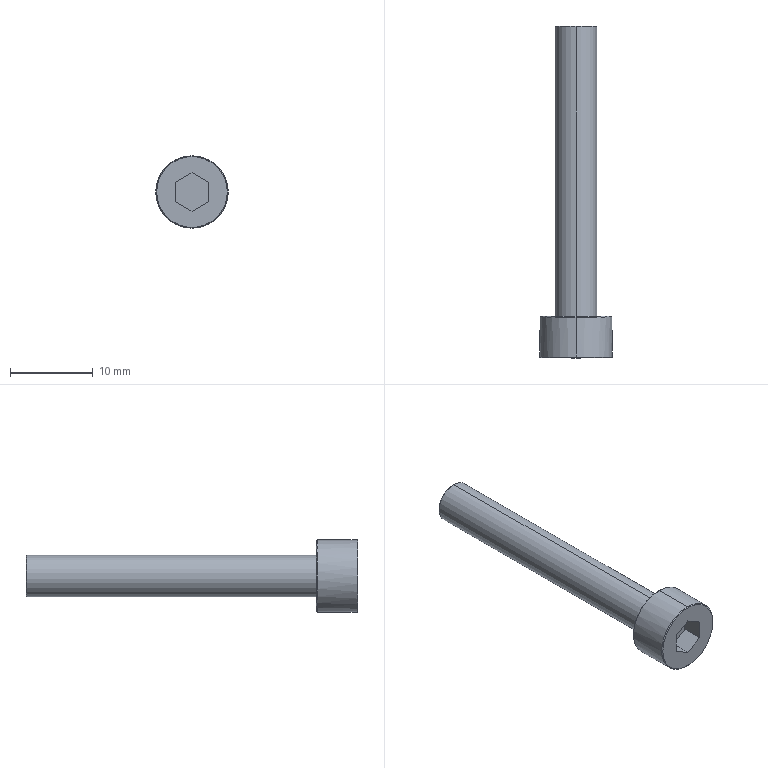Part | SolidWorks | features BaseBody 1 | 1 solid | 20 faces | box 8.72 x 40 x 8.72 mm | volume 950.488 mm3 | plane 10 | cone 6 | cylinder 4 | commonest cylinder face diameters 5 x2 8.72 x2
STEP:
#1=CARTESIAN_POINT('',(0.,39.9,-2.5));
#2=VERTEX_POINT('',#1);
#3=CARTESIAN_POINT('',(0.,39.9,2.5));
#4=VERTEX_POINT('',#3);
#5=CARTESIAN_POINT('',(0.,39.9,0.));
#6=DIRECTION('',(0.,-1.,0.));
#7=DIRECTION('',(0.,0.,-1.));
#8=AXIS2_PLACEMENT_3D('',#5,#6,#7);
#9=CIRCLE('',#8,2.5);
#10=EDGE_CURVE('',#2,#4,#9,.T.);
#11=ORIENTED_EDGE('',*,*,#10,.T.);
#12=CARTESIAN_POINT('',(0.,5.,2.5));
#13=VERTEX_POINT('',#12);
#14=CARTESIAN_POINT('',(0.,40.,2.5));
#15=DIRECTION('',(0.,-1.,0.));
#16=VECTOR('',#15,1000.);
#17=LINE('',#14,#16);
#18=EDGE_CURVE('',#4,#13,#17,.T.);
#19=ORIENTED_EDGE('',*,*,#18,.T.);
#20=CARTESIAN_POINT('',(0.,5.,-2.5));
#21=VERTEX_POINT('',#20);
#22=CARTESIAN_POINT('',(0.,5.,0.));
#23=DIRECTION('',(0.,1.,0.));
#24=DIRECTION('',(0.,0.,-1.));
#25=AXIS2_PLACEMENT_3D('',#22,#23,#24);
#26=CIRCLE('',#25,2.5);
#27=EDGE_CURVE('',#13,#21,#26,.T.);
#28=ORIENTED_EDGE('',*,*,#27,.T.);
#29=CARTESIAN_POINT('',(0.,40.,-2.5));
#30=DIRECTION('',(0.,-1.,0.));
#31=VECTOR('',#30,1000.);
#32=LINE('',#29,#31);
#33=EDGE_CURVE('',#2,#21,#32,.T.);
#34=ORIENTED_EDGE('',*,*,#33,.F.);
#35=EDGE_LOOP('',(#11,#19,#28,#34));
#36=FACE_OUTER_BOUND('',#35,.T.);
#37=CARTESIAN_POINT('',(0.,40.,0.));
#38=DIRECTION('',(0.,-1.,0.));
#39=DIRECTION('',(0.,0.,-1.));
#40=AXIS2_PLACEMENT_3D('',#37,#38,#39);
#41=CYLINDRICAL_SURFACE('',#40,2.5);
#42=ADVANCED_FACE('',(#36),#41,.T.);
#43=CARTESIAN_POINT('',(0.,40.,-2.4));
#44=VERTEX_POINT('',#43);
#45=CARTESIAN_POINT('',(0.,40.,2.4));
#46=VERTEX_POINT('',#45);
#47=CARTESIAN_POINT('',(0.,40.,0.));
#48=DIRECTION('',(0.,-1.,0.));
#49=DIRECTION('',(0.,0.,-1.));
#50=AXIS2_PLACEMENT_3D('',#47,#48,#49);
#51=CIRCLE('',#50,2.4);
#52=EDGE_CURVE('',#44,#46,#51,.T.);
#53=ORIENTED_EDGE('',*,*,#52,.T.);
#54=CARTESIAN_POINT('',(0.,39.9,2.5));
#55=DIRECTION('',(0.,-0.7071,0.7071));
#56=VECTOR('',#55,1000.);
#57=LINE('',#54,#56);
#58=EDGE_CURVE('',#46,#4,#57,.T.);
#59=ORIENTED_EDGE('',*,*,#58,.T.);
#60=ORIENTED_EDGE('',*,*,#10,.F.);
#61=CARTESIAN_POINT('',(0.,39.9,-2.5));
#62=DIRECTION('',(0.,-0.7071,-0.7071));
#63=VECTOR('',#62,1000.);
#64=LINE('',#61,#63);
#65=EDGE_CURVE('',#44,#2,#64,.T.);
#66=ORIENTED_EDGE('',*,*,#65,.F.);
#67=EDGE_LOOP('',(#53,#59,#60,#66));
#68=FACE_OUTER_BOUND('',#67,.T.);
#69=CARTESIAN_POINT('',(0.,39.9,0.));
#70=DIRECTION('',(0.,-1.,0.));
#71=DIRECTION('',(0.,0.,-1.));
#72=AXIS2_PLACEMENT_3D('',#69,#70,#71);
#73=CONICAL_SURFACE('',#72,2.5,0.7854);
#74=ADVANCED_FACE('',(#68),#73,.T.);
#75=CARTESIAN_POINT('',(0.,5.,4.26));
#76=VERTEX_POINT('',#75);
#77=CARTESIAN_POINT('',(0.,5.,-4.26));
#78=VERTEX_POINT('',#77);
#79=CARTESIAN_POINT('',(0.,5.,0.));
#80=DIRECTION('',(0.,1.,0.));
#81=DIRECTION('',(0.,0.,-1.));
#82=AXIS2_PLACEMENT_3D('',#79,#80,#81);
#83=CIRCLE('',#82,4.26);
#84=EDGE_CURVE('',#76,#78,#83,.T.);
#85=ORIENTED_EDGE('',*,*,#84,.F.);
#86=CARTESIAN_POINT('',(0.,4.9,4.36));
#87=VERTEX_POINT('',#86);
#88=CARTESIAN_POINT('',(0.,4.9,4.36));
#89=DIRECTION('',(0.,-0.7071,0.7071));
#90=VECTOR('',#89,1000.);
#91=LINE('',#88,#90);
#92=EDGE_CURVE('',#76,#87,#91,.T.);
#93=ORIENTED_EDGE('',*,*,#92,.T.);
#94=CARTESIAN_POINT('',(0.,4.9,-4.36));
#95=VERTEX_POINT('',#94);
#96=CARTESIAN_POINT('',(0.,4.9,0.));
#97=DIRECTION('',(0.,1.,0.));
#98=DIRECTION('',(0.,0.,-1.));
#99=AXIS2_PLACEMENT_3D('',#96,#97,#98);
#100=CIRCLE('',#99,4.36);
#101=EDGE_CURVE('',#87,#95,#100,.T.);
#102=ORIENTED_EDGE('',*,*,#101,.T.);
#103=CARTESIAN_POINT('',(0.,4.9,-4.36));
#104=DIRECTION('',(0.,-0.7071,-0.7071));
#105=VECTOR('',#104,1000.);
#106=LINE('',#103,#105);
#107=EDGE_CURVE('',#78,#95,#106,.T.);
#108=ORIENTED_EDGE('',*,*,#107,.F.);
#109=EDGE_LOOP('',(#85,#93,#102,#108));
#110=FACE_OUTER_BOUND('',#109,.T.);
#111=CARTESIAN_POINT('',(0.,4.9,0.));
#112=DIRECTION('',(0.,-1.,0.));
#113=DIRECTION('',(0.,0.,-1.));
#114=AXIS2_PLACEMENT_3D('',#111,#112,#113);
#115=CONICAL_SURFACE('',#114,4.36,0.7854);
#116=ADVANCED_FACE('',(#110),#115,.T.);
#117=ORIENTED_EDGE('',*,*,#101,.F.);
#118=CARTESIAN_POINT('',(0.,0.1,4.36));
#119=VERTEX_POINT('',#118);
#120=CARTESIAN_POINT('',(0.,5.,4.36));
#121=DIRECTION('',(0.,-1.,0.));
#122=VECTOR('',#121,1000.);
#123=LINE('',#120,#122);
#124=EDGE_CURVE('',#87,#119,#123,.T.);
#125=ORIENTED_EDGE('',*,*,#124,.T.);
#126=CARTESIAN_POINT('',(4.36,0.1,0.));
#127=VERTEX_POINT('',#126);
#128=CARTESIAN_POINT('',(0.,0.1,0.));
#129=DIRECTION('',(0.,1.,0.));
#130=DIRECTION('',(0.,0.,-1.));
#131=AXIS2_PLACEMENT_3D('',#128,#129,#130);
#132=CIRCLE('',#131,4.36);
#133=EDGE_CURVE('',#119,#127,#132,.T.);
#134=ORIENTED_EDGE('',*,*,#133,.T.);
#135=CARTESIAN_POINT('',(0.,0.1,-4.36));
#136=VERTEX_POINT('',#135);
#137=CARTESIAN_POINT('',(0.,0.1,0.));
#138=DIRECTION('',(0.,1.,0.));
#139=DIRECTION('',(0.,0.,-1.));
#140=AXIS2_PLACEMENT_3D('',#137,#138,#139);
#141=CIRCLE('',#140,4.36);
#142=EDGE_CURVE('',#127,#136,#141,.T.);
#143=ORIENTED_EDGE('',*,*,#142,.T.);
#144=CARTESIAN_POINT('',(0.,5.,-4.36));
#145=DIRECTION('',(0.,-1.,0.));
#146=VECTOR('',#145,1000.);
#147=LINE('',#144,#146);
#148=EDGE_CURVE('',#95,#136,#147,.T.);
#149=ORIENTED_EDGE('',*,*,#148,.F.);
#150=EDGE_LOOP('',(#117,#125,#134,#143,#149));
#151=FACE_OUTER_BOUND('',#150,.T.);
#152=CARTESIAN_POINT('',(0.,5.,0.));
#153=DIRECTION('',(0.,-1.,0.));
#154=DIRECTION('',(0.,0.,-1.));
#155=AXIS2_PLACEMENT_3D('',#152,#153,#154);
#156=CYLINDRICAL_SURFACE('',#155,4.36);
#157=ADVANCED_FACE('',(#151),#156,.T.);
#158=CARTESIAN_POINT('',(-4.26,0.,0.));
#159=VERTEX_POINT('',#158);
#160=CARTESIAN_POINT('',(4.26,0.,0.));
#161=VERTEX_POINT('',#160);
#162=CARTESIAN_POINT('',(0.,0.,0.));
#163=DIRECTION('',(0.,1.,0.));
#164=DIRECTION('',(-1.,0.,0.));
#165=AXIS2_PLACEMENT_3D('',#162,#163,#164);
#166=CIRCLE('',#165,4.26);
#167=EDGE_CURVE('',#159,#161,#166,.T.);
#168=ORIENTED_EDGE('',*,*,#167,.T.);
#169=CARTESIAN_POINT('',(4.36,0.1,0.));
#170=DIRECTION('',(0.7071,0.7071,0.));
#171=VECTOR('',#170,1000.);
#172=LINE('',#169,#171);
#173=EDGE_CURVE('',#161,#127,#172,.T.);
#174=ORIENTED_EDGE('',*,*,#173,.T.);
#175=ORIENTED_EDGE('',*,*,#133,.F.);
#176=CARTESIAN_POINT('',(-4.36,0.1,0.));
#177=VERTEX_POINT('',#176);
#178=CARTESIAN_POINT('',(0.,0.1,0.));
#179=DIRECTION('',(0.,1.,0.));
#180=DIRECTION('',(0.,0.,-1.));
#181=AXIS2_PLACEMENT_3D('',#178,#179,#180);
#182=CIRCLE('',#181,4.36);
#183=EDGE_CURVE('',#177,#119,#182,.T.);
#184=ORIENTED_EDGE('',*,*,#183,.F.);
#185=CARTESIAN_POINT('',(-4.36,0.1,0.));
#186=DIRECTION('',(-0.7071,0.7071,0.));
#187=VECTOR('',#186,1000.);
#188=LINE('',#185,#187);
#189=EDGE_CURVE('',#159,#177,#188,.T.);
#190=ORIENTED_EDGE('',*,*,#189,.F.);
#191=EDGE_LOOP('',(#168,#174,#175,#184,#190));
#192=FACE_OUTER_BOUND('',#191,.T.);
#193=CARTESIAN_POINT('',(0.,0.1,0.));
#194=DIRECTION('',(0.,1.,0.));
#195=DIRECTION('',(-1.,0.,0.));
#196=AXIS2_PLACEMENT_3D('',#193,#194,#195);
#197=CONICAL_SURFACE('',#196,4.36,0.7854);
#198=ADVANCED_FACE('',(#192),#197,.T.);
#199=ORIENTED_EDGE('',*,*,#18,.F.);
#200=CARTESIAN_POINT('',(0.,39.9,0.));
#201=DIRECTION('',(0.,-1.,0.));
#202=DIRECTION('',(0.,0.,-1.));
#203=AXIS2_PLACEMENT_3D('',#200,#201,#202);
#204=CIRCLE('',#203,2.5);
#205=EDGE_CURVE('',#4,#2,#204,.T.);
#206=ORIENTED_EDGE('',*,*,#205,.T.);
#207=ORIENTED_EDGE('',*,*,#33,.T.);
#208=CARTESIAN_POINT('',(0.,5.,0.));
#209=DIRECTION('',(0.,1.,0.));
#210=DIRECTION('',(0.,0.,-1.));
#211=AXIS2_PLACEMENT_3D('',#208,#209,#210);
#212=CIRCLE('',#211,2.5);
#213=EDGE_CURVE('',#21,#13,#212,.T.);
#214=ORIENTED_EDGE('',*,*,#213,.T.);
#215=EDGE_LOOP('',(#199,#206,#207,#214));
#216=FACE_OUTER_BOUND('',#215,.T.);
#217=CARTESIAN_POINT('',(0.,40.,0.));
#218=DIRECTION('',(0.,-1.,0.));
#219=DIRECTION('',(0.,0.,-1.));
#220=AXIS2_PLACEMENT_3D('',#217,#218,#219);
#221=CYLINDRICAL_SURFACE('',#220,2.5);
#222=ADVANCED_FACE('',(#216),#221,.T.);
#223=ORIENTED_EDGE('',*,*,#213,.F.);
#224=ORIENTED_EDGE('',*,*,#27,.F.);
#225=EDGE_LOOP('',(#223,#224));
#226=FACE_BOUND('',#225,.T.);
#227=CARTESIAN_POINT('',(0.,5.,0.));
#228=DIRECTION('',(0.,1.,0.));
#229=DIRECTION('',(0.,0.,-1.));
#230=AXIS2_PLACEMENT_3D('',#227,#228,#229);
#231=CIRCLE('',#230,4.26);
#232=EDGE_CURVE('',#78,#76,#231,.T.);
#233=ORIENTED_EDGE('',*,*,#232,.T.);
#234=ORIENTED_EDGE('',*,*,#84,.T.);
#235=EDGE_LOOP('',(#233,#234));
#236=FACE_OUTER_BOUND('',#235,.T.);
#237=CARTESIAN_POINT('',(0.,5.,0.));
#238=DIRECTION('',(0.,1.,0.));
#239=DIRECTION('',(0.,0.,1.));
#240=AXIS2_PLACEMENT_3D('',#237,#238,#239);
#241=PLANE('',#240);
#242=ADVANCED_FACE('',(#226,#236),#241,.T.);
#243=ORIENTED_EDGE('',*,*,#58,.F.);
#244=CARTESIAN_POINT('',(0.,40.,0.));
#245=DIRECTION('',(0.,-1.,0.));
#246=DIRECTION('',(0.,0.,-1.));
#247=AXIS2_PLACEMENT_3D('',#244,#245,#246);
#248=CIRCLE('',#247,2.4);
#249=EDGE_CURVE('',#46,#44,#248,.T.);
#250=ORIENTED_EDGE('',*,*,#249,.T.);
#251=ORIENTED_EDGE('',*,*,#65,.T.);
#252=ORIENTED_EDGE('',*,*,#205,.F.);
#253=EDGE_LOOP('',(#243,#250,#251,#252));
#254=FACE_OUTER_BOUND('',#253,.T.);
#255=CARTESIAN_POINT('',(0.,39.9,0.));
#256=DIRECTION('',(0.,-1.,0.));
#257=DIRECTION('',(0.,0.,-1.));
#258=AXIS2_PLACEMENT_3D('',#255,#256,#257);
#259=CONICAL_SURFACE('',#258,2.5,0.7854);
#260=ADVANCED_FACE('',(#254),#259,.T.);
#261=ORIENTED_EDGE('',*,*,#92,.F.);
#262=ORIENTED_EDGE('',*,*,#232,.F.);
#263=ORIENTED_EDGE('',*,*,#107,.T.);
#264=CARTESIAN_POINT('',(0.,4.9,0.));
#265=DIRECTION('',(0.,1.,0.));
#266=DIRECTION('',(0.,0.,-1.));
#267=AXIS2_PLACEMENT_3D('',#264,#265,#266);
#268=CIRCLE('',#267,4.36);
#269=EDGE_CURVE('',#95,#87,#268,.T.);
#270=ORIENTED_EDGE('',*,*,#269,.T.);
#271=EDGE_LOOP('',(#261,#262,#263,#270));
#272=FACE_OUTER_BOUND('',#271,.T.);
#273=CARTESIAN_POINT('',(0.,4.9,0.));
#274=DIRECTION('',(0.,-1.,0.));
#275=DIRECTION('',(0.,0.,-1.));
#276=AXIS2_PLACEMENT_3D('',#273,#274,#275);
#277=CONICAL_SURFACE('',#276,4.36,0.7854);
#278=ADVANCED_FACE('',(#272),#277,.T.);
#279=ORIENTED_EDGE('',*,*,#52,.F.);
#280=ORIENTED_EDGE('',*,*,#249,.F.);
#281=EDGE_LOOP('',(#279,#280));
#282=FACE_OUTER_BOUND('',#281,.T.);
#283=CARTESIAN_POINT('',(0.,40.,0.));
#284=DIRECTION('',(0.,1.,0.));
#285=DIRECTION('',(0.,0.,1.));
#286=AXIS2_PLACEMENT_3D('',#283,#284,#285);
#287=PLANE('',#286);
#288=ADVANCED_FACE('',(#282),#287,.T.);
#289=ORIENTED_EDGE('',*,*,#124,.F.);
#290=ORIENTED_EDGE('',*,*,#269,.F.);
#291=ORIENTED_EDGE('',*,*,#148,.T.);
#292=CARTESIAN_POINT('',(0.,0.1,0.));
#293=DIRECTION('',(0.,1.,0.));
#294=DIRECTION('',(0.,0.,-1.));
#295=AXIS2_PLACEMENT_3D('',#292,#293,#294);
#296=CIRCLE('',#295,4.36);
#297=EDGE_CURVE('',#136,#177,#296,.T.);
#298=ORIENTED_EDGE('',*,*,#297,.T.);
#299=ORIENTED_EDGE('',*,*,#183,.T.);
#300=EDGE_LOOP('',(#289,#290,#291,#298,#299));
#301=FACE_OUTER_BOUND('',#300,.T.);
#302=CARTESIAN_POINT('',(0.,5.,0.));
#303=DIRECTION('',(0.,-1.,0.));
#304=DIRECTION('',(0.,0.,-1.));
#305=AXIS2_PLACEMENT_3D('',#302,#303,#304);
#306=CYLINDRICAL_SURFACE('',#305,4.36);
#307=ADVANCED_FACE('',(#301),#306,.T.);
#308=ORIENTED_EDGE('',*,*,#173,.F.);
#309=CARTESIAN_POINT('',(0.,0.,0.));
#310=DIRECTION('',(0.,1.,0.));
#311=DIRECTION('',(-1.,0.,0.));
#312=AXIS2_PLACEMENT_3D('',#309,#310,#311);
#313=CIRCLE('',#312,4.26);
#314=EDGE_CURVE('',#161,#159,#313,.T.);
#315=ORIENTED_EDGE('',*,*,#314,.T.);
#316=ORIENTED_EDGE('',*,*,#189,.T.);
#317=ORIENTED_EDGE('',*,*,#297,.F.);
#318=ORIENTED_EDGE('',*,*,#142,.F.);
#319=EDGE_LOOP('',(#308,#315,#316,#317,#318));
#320=FACE_OUTER_BOUND('',#319,.T.);
#321=CARTESIAN_POINT('',(0.,0.1,0.));
#322=DIRECTION('',(0.,1.,0.));
#323=DIRECTION('',(-1.,0.,0.));
#324=AXIS2_PLACEMENT_3D('',#321,#322,#323);
#325=CONICAL_SURFACE('',#324,4.36,0.7854);
#326=ADVANCED_FACE('',(#320),#325,.T.);
#327=CARTESIAN_POINT('',(0.,0.,-2.321));
#328=VERTEX_POINT('',#327);
#329=CARTESIAN_POINT('',(2.01,0.,-1.16));
#330=VERTEX_POINT('',#329);
#331=CARTESIAN_POINT('',(0.,0.,-2.321));
#332=DIRECTION('',(0.866,0.,0.5));
#333=VECTOR('',#332,1000.);
#334=LINE('',#331,#333);
#335=EDGE_CURVE('',#328,#330,#334,.T.);
#336=ORIENTED_EDGE('',*,*,#335,.F.);
#337=CARTESIAN_POINT('',(-2.01,0.,-1.16));
#338=VERTEX_POINT('',#337);
#339=CARTESIAN_POINT('',(-2.01,0.,-1.16));
#340=DIRECTION('',(0.866,0.,-0.5));
#341=VECTOR('',#340,1000.);
#342=LINE('',#339,#341);
#343=EDGE_CURVE('',#338,#328,#342,.T.);
#344=ORIENTED_EDGE('',*,*,#343,.F.);
#345=CARTESIAN_POINT('',(-2.01,0.,1.16));
#346=VERTEX_POINT('',#345);
#347=CARTESIAN_POINT('',(-2.01,0.,0.));
#348=DIRECTION('',(0.,0.,-1.));
#349=VECTOR('',#348,1000.);
#350=LINE('',#347,#349);
#351=EDGE_CURVE('',#346,#338,#350,.T.);
#352=ORIENTED_EDGE('',*,*,#351,.F.);
#353=CARTESIAN_POINT('',(0.,0.,2.321));
#354=VERTEX_POINT('',#353);
#355=CARTESIAN_POINT('',(0.,0.,2.321));
#356=DIRECTION('',(-0.866,0.,-0.5));
#357=VECTOR('',#356,1000.);
#358=LINE('',#355,#357);
#359=EDGE_CURVE('',#354,#346,#358,.T.);
#360=ORIENTED_EDGE('',*,*,#359,.F.);
#361=CARTESIAN_POINT('',(2.01,0.,1.16));
#362=VERTEX_POINT('',#361);
#363=CARTESIAN_POINT('',(2.01,0.,1.16));
#364=DIRECTION('',(-0.866,0.,0.5));
#365=VECTOR('',#364,1000.);
#366=LINE('',#363,#365);
#367=EDGE_CURVE('',#362,#354,#366,.T.);
#368=ORIENTED_EDGE('',*,*,#367,.F.);
#369=CARTESIAN_POINT('',(2.01,0.,0.));
#370=DIRECTION('',(0.,0.,1.));
#371=VECTOR('',#370,1000.);
#372=LINE('',#369,#371);
#373=EDGE_CURVE('',#330,#362,#372,.T.);
#374=ORIENTED_EDGE('',*,*,#373,.F.);
#375=EDGE_LOOP('',(#336,#344,#352,#360,#368,#374));
#376=FACE_BOUND('',#375,.T.);
#377=ORIENTED_EDGE('',*,*,#167,.F.);
#378=ORIENTED_EDGE('',*,*,#314,.F.);
#379=EDGE_LOOP('',(#377,#378));
#380=FACE_OUTER_BOUND('',#379,.T.);
#381=CARTESIAN_POINT('',(0.,0.,0.));
#382=DIRECTION('',(0.,1.,0.));
#383=DIRECTION('',(0.,0.,1.));
#384=AXIS2_PLACEMENT_3D('',#381,#382,#383);
#385=PLANE('',#384);
#386=ADVANCED_FACE('',(#376,#380),#385,.F.);
#387=CARTESIAN_POINT('',(2.01,2.5,1.16));
#388=VERTEX_POINT('',#387);
#389=CARTESIAN_POINT('',(2.01,2.5,1.16));
#390=DIRECTION('',(0.,-1.,0.));
#391=VECTOR('',#390,1000.);
#392=LINE('',#389,#391);
#393=EDGE_CURVE('',#388,#362,#392,.T.);
#394=ORIENTED_EDGE('',*,*,#393,.F.);
#395=CARTESIAN_POINT('',(2.01,2.5,-1.16));
#396=VERTEX_POINT('',#395);
#397=CARTESIAN_POINT('',(2.01,2.5,-1.16));
#398=DIRECTION('',(0.,0.,1.));
#399=VECTOR('',#398,1000.);
#400=LINE('',#397,#399);
#401=EDGE_CURVE('',#396,#388,#400,.T.);
#402=ORIENTED_EDGE('',*,*,#401,.F.);
#403=CARTESIAN_POINT('',(2.01,2.5,-1.16));
#404=DIRECTION('',(0.,1.,0.));
#405=VECTOR('',#404,1000.);
#406=LINE('',#403,#405);
#407=EDGE_CURVE('',#330,#396,#406,.T.);
#408=ORIENTED_EDGE('',*,*,#407,.F.);
#409=ORIENTED_EDGE('',*,*,#373,.T.);
#410=EDGE_LOOP('',(#394,#402,#408,#409));
#411=FACE_OUTER_BOUND('',#410,.T.);
#412=CARTESIAN_POINT('',(2.01,2.5,-1.16));
#413=DIRECTION('',(1.,0.,0.));
#414=DIRECTION('',(0.,0.,-1.));
#415=AXIS2_PLACEMENT_3D('',#412,#413,#414);
#416=PLANE('',#415);
#417=ADVANCED_FACE('',(#411),#416,.F.);
#418=ORIENTED_EDGE('',*,*,#407,.T.);
#419=CARTESIAN_POINT('',(0.,2.5,-2.321));
#420=VERTEX_POINT('',#419);
#421=CARTESIAN_POINT('',(0.,2.5,-2.321));
#422=DIRECTION('',(0.866,0.,0.5));
#423=VECTOR('',#422,1000.);
#424=LINE('',#421,#423);
#425=EDGE_CURVE('',#420,#396,#424,.T.);
#426=ORIENTED_EDGE('',*,*,#425,.F.);
#427=CARTESIAN_POINT('',(0.,2.5,-2.321));
#428=DIRECTION('',(0.,1.,0.));
#429=VECTOR('',#428,1000.);
#430=LINE('',#427,#429);
#431=EDGE_CURVE('',#328,#420,#430,.T.);
#432=ORIENTED_EDGE('',*,*,#431,.F.);
#433=ORIENTED_EDGE('',*,*,#335,.T.);
#434=EDGE_LOOP('',(#418,#426,#432,#433));
#435=FACE_OUTER_BOUND('',#434,.T.);
#436=CARTESIAN_POINT('',(0.,2.5,-2.321));
#437=DIRECTION('',(0.5,0.,-0.866));
#438=DIRECTION('',(-0.866,0.,-0.5));
#439=AXIS2_PLACEMENT_3D('',#436,#437,#438);
#440=PLANE('',#439);
#441=ADVANCED_FACE('',(#435),#440,.F.);
#442=ORIENTED_EDGE('',*,*,#431,.T.);
#443=CARTESIAN_POINT('',(-2.01,2.5,-1.16));
#444=VERTEX_POINT('',#443);
#445=CARTESIAN_POINT('',(-2.01,2.5,-1.16));
#446=DIRECTION('',(0.866,0.,-0.5));
#447=VECTOR('',#446,1000.);
#448=LINE('',#445,#447);
#449=EDGE_CURVE('',#444,#420,#448,.T.);
#450=ORIENTED_EDGE('',*,*,#449,.F.);
#451=CARTESIAN_POINT('',(-2.01,2.5,-1.16));
#452=DIRECTION('',(0.,1.,0.));
#453=VECTOR('',#452,1000.);
#454=LINE('',#451,#453);
#455=EDGE_CURVE('',#338,#444,#454,.T.);
#456=ORIENTED_EDGE('',*,*,#455,.F.);
#457=ORIENTED_EDGE('',*,*,#343,.T.);
#458=EDGE_LOOP('',(#442,#450,#456,#457));
#459=FACE_OUTER_BOUND('',#458,.T.);
#460=CARTESIAN_POINT('',(-2.01,2.5,-1.16));
#461=DIRECTION('',(-0.5,0.,-0.866));
#462=DIRECTION('',(-0.866,0.,0.5));
#463=AXIS2_PLACEMENT_3D('',#460,#461,#462);
#464=PLANE('',#463);
#465=ADVANCED_FACE('',(#459),#464,.F.);
#466=ORIENTED_EDGE('',*,*,#455,.T.);
#467=CARTESIAN_POINT('',(-2.01,2.5,1.16));
#468=VERTEX_POINT('',#467);
#469=CARTESIAN_POINT('',(-2.01,2.5,1.16));
#470=DIRECTION('',(0.,0.,-1.));
#471=VECTOR('',#470,1000.);
#472=LINE('',#469,#471);
#473=EDGE_CURVE('',#468,#444,#472,.T.);
#474=ORIENTED_EDGE('',*,*,#473,.F.);
#475=CARTESIAN_POINT('',(-2.01,2.5,1.16));
#476=DIRECTION('',(0.,1.,0.));
#477=VECTOR('',#476,1000.);
#478=LINE('',#475,#477);
#479=EDGE_CURVE('',#346,#468,#478,.T.);
#480=ORIENTED_EDGE('',*,*,#479,.F.);
#481=ORIENTED_EDGE('',*,*,#351,.T.);
#482=EDGE_LOOP('',(#466,#474,#480,#481));
#483=FACE_OUTER_BOUND('',#482,.T.);
#484=CARTESIAN_POINT('',(-2.01,2.5,1.16));
#485=DIRECTION('',(-1.,0.,0.));
#486=DIRECTION('',(0.,0.,1.));
#487=AXIS2_PLACEMENT_3D('',#484,#485,#486);
#488=PLANE('',#487);
#489=ADVANCED_FACE('',(#483),#488,.F.);
#490=ORIENTED_EDGE('',*,*,#479,.T.);
#491=CARTESIAN_POINT('',(0.,2.5,2.321));
#492=VERTEX_POINT('',#491);
#493=CARTESIAN_POINT('',(0.,2.5,2.321));
#494=DIRECTION('',(-0.866,0.,-0.5));
#495=VECTOR('',#494,1000.);
#496=LINE('',#493,#495);
#497=EDGE_CURVE('',#492,#468,#496,.T.);
#498=ORIENTED_EDGE('',*,*,#497,.F.);
#499=CARTESIAN_POINT('',(0.,2.5,2.321));
#500=DIRECTION('',(0.,1.,0.));
#501=VECTOR('',#500,1000.);
#502=LINE('',#499,#501);
#503=EDGE_CURVE('',#354,#492,#502,.T.);
#504=ORIENTED_EDGE('',*,*,#503,.F.);
#505=ORIENTED_EDGE('',*,*,#359,.T.);
#506=EDGE_LOOP('',(#490,#498,#504,#505));
#507=FACE_OUTER_BOUND('',#506,.T.);
#508=CARTESIAN_POINT('',(0.,2.5,2.321));
#509=DIRECTION('',(-0.5,0.,0.866));
#510=DIRECTION('',(0.866,0.,0.5));
#511=AXIS2_PLACEMENT_3D('',#508,#509,#510);
#512=PLANE('',#511);
#513=ADVANCED_FACE('',(#507),#512,.F.);
#514=ORIENTED_EDGE('',*,*,#503,.T.);
#515=CARTESIAN_POINT('',(2.01,2.5,1.16));
#516=DIRECTION('',(-0.866,0.,0.5));
#517=VECTOR('',#516,1000.);
#518=LINE('',#515,#517);
#519=EDGE_CURVE('',#388,#492,#518,.T.);
#520=ORIENTED_EDGE('',*,*,#519,.F.);
#521=ORIENTED_EDGE('',*,*,#393,.T.);
#522=ORIENTED_EDGE('',*,*,#367,.T.);
#523=EDGE_LOOP('',(#514,#520,#521,#522));
#524=FACE_OUTER_BOUND('',#523,.T.);
#525=CARTESIAN_POINT('',(2.01,2.5,1.16));
#526=DIRECTION('',(0.5,0.,0.866));
#527=DIRECTION('',(0.866,0.,-0.5));
#528=AXIS2_PLACEMENT_3D('',#525,#526,#527);
#529=PLANE('',#528);
#530=ADVANCED_FACE('',(#524),#529,.F.);
#531=ORIENTED_EDGE('',*,*,#473,.T.);
#532=ORIENTED_EDGE('',*,*,#449,.T.);
#533=ORIENTED_EDGE('',*,*,#425,.T.);
#534=ORIENTED_EDGE('',*,*,#401,.T.);
#535=ORIENTED_EDGE('',*,*,#519,.T.);
#536=ORIENTED_EDGE('',*,*,#497,.T.);
#537=EDGE_LOOP('',(#531,#532,#533,#534,#535,#536));
#538=FACE_OUTER_BOUND('',#537,.T.);
#539=CARTESIAN_POINT('',(0.,2.5,0.));
#540=DIRECTION('',(0.,-1.,0.));
#541=DIRECTION('',(0.,0.,-1.));
#542=AXIS2_PLACEMENT_3D('',#539,#540,#541);
#543=PLANE('',#542);
#544=ADVANCED_FACE('',(#538),#543,.T.);
#545=CLOSED_SHELL('',(#42,#74,#116,#157,#198,#222,#242,#260,#278,#288,#307,#326,#386,#417,#441,#465,#489,#513,#530,#544));
#546=MANIFOLD_SOLID_BREP('',#545);
#547=CARTESIAN_POINT('',(0.,0.,0.));
#548=DIRECTION('',(0.,0.,1.));
#549=DIRECTION('',(1.,0.,0.));
#550=AXIS2_PLACEMENT_3D('',#547,#548,#549);
#551=(LENGTH_UNIT()NAMED_UNIT(*)SI_UNIT(.MILLI.,.METRE.));
#552=UNCERTAINTY_MEASURE_WITH_UNIT(LENGTH_MEASURE(0.00001),#551,'','');
#553=(NAMED_UNIT(*)PLANE_ANGLE_UNIT()SI_UNIT($,.RADIAN.));
#554=(NAMED_UNIT(*)SI_UNIT($,.STERADIAN.)SOLID_ANGLE_UNIT());
#555=(GEOMETRIC_REPRESENTATION_CONTEXT(3)GLOBAL_UNCERTAINTY_ASSIGNED_CONTEXT((#552))GLOBAL_UNIT_ASSIGNED_CONTEXT((#551,#553,#554))REPRESENTATION_CONTEXT('',''));
#556=ADVANCED_BREP_SHAPE_REPRESENTATION('',(#546,#550),#555);